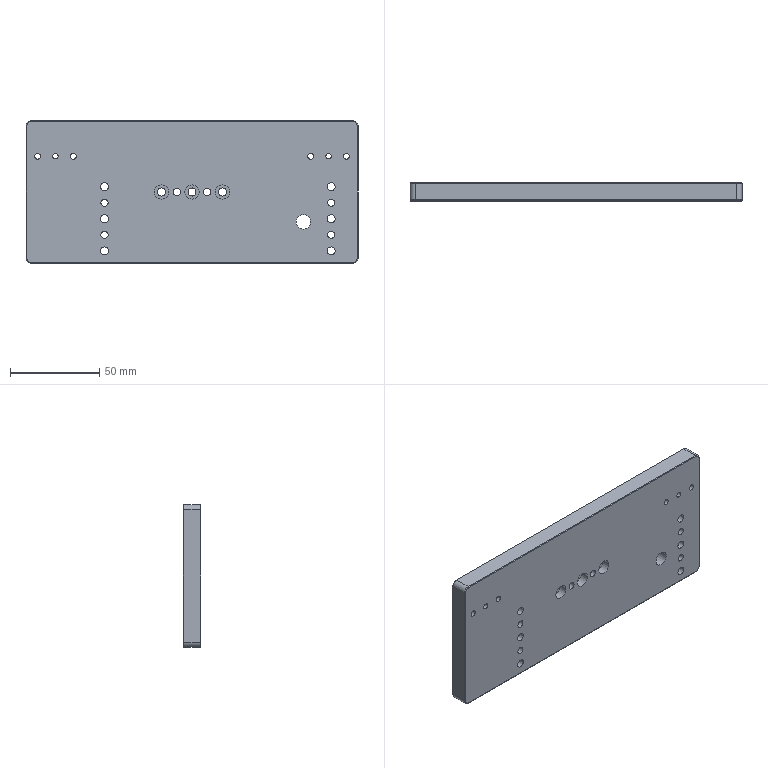Part | 1 solid | 70 faces | box 186 x 10 x 80 mm | volume 143846 mm3 | cylinder 37 | plane 25 | cone 8 | commonest cylinder face diameters 8 x10 4.5 x9 4 x6 3.3 x4 6 x4 3 x2